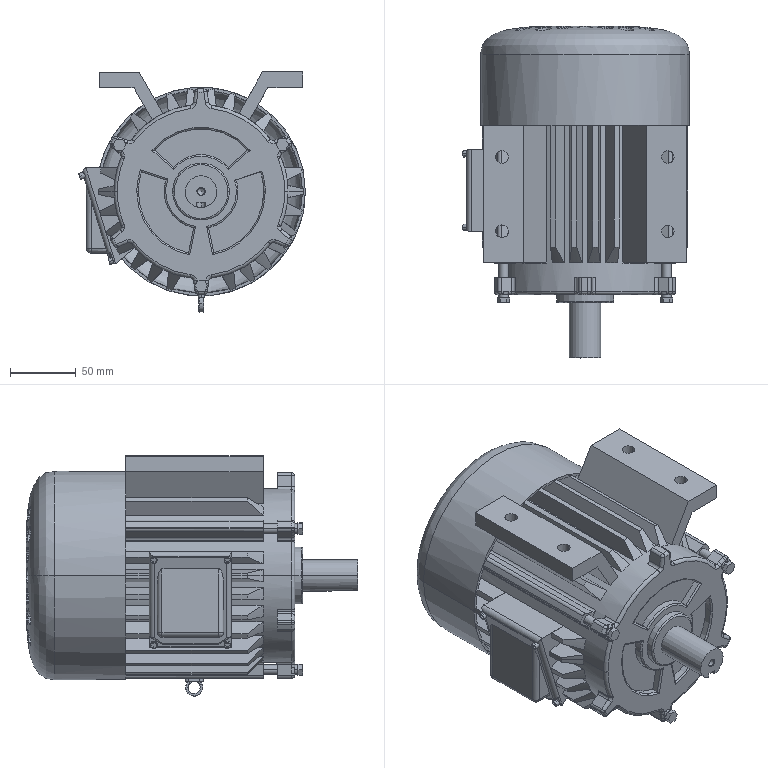Part | NX | features BREP 1, HOLE PACKAGE 1, OFFSET 1, SCALE 1, SIMPLE HOLE 1, SYMBOLIC_THREAD 1 | 1 solid | 652 faces | volume 2573797 mm3 | cylinder 300 | plane 229 | torus 55 | cone 26 | spline 26 | sphere 16 | commonest cylinder face diameters 4.8 x102 12 x80 156 x40 2.4 x14 7.238 x12 7.2 x10